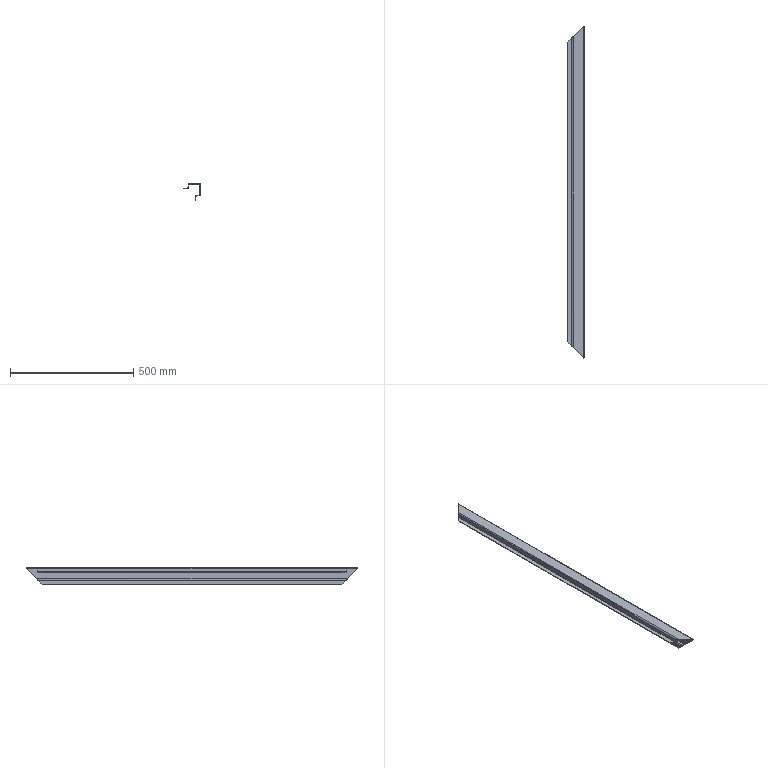Part | SolidWorks | features EdgeFlange 5, ICE 2, Extrusion 1, FlatPattern 1, SheetMetal 1, SolidToSheetMetal 1 | 1 solid | 48 faces | box 68 x 1349 x 68 mm | volume 418242 mm3 | plane 26 | spline 12 | cylinder 10 | commonest cylinder face diameters 4 x5 8 x5